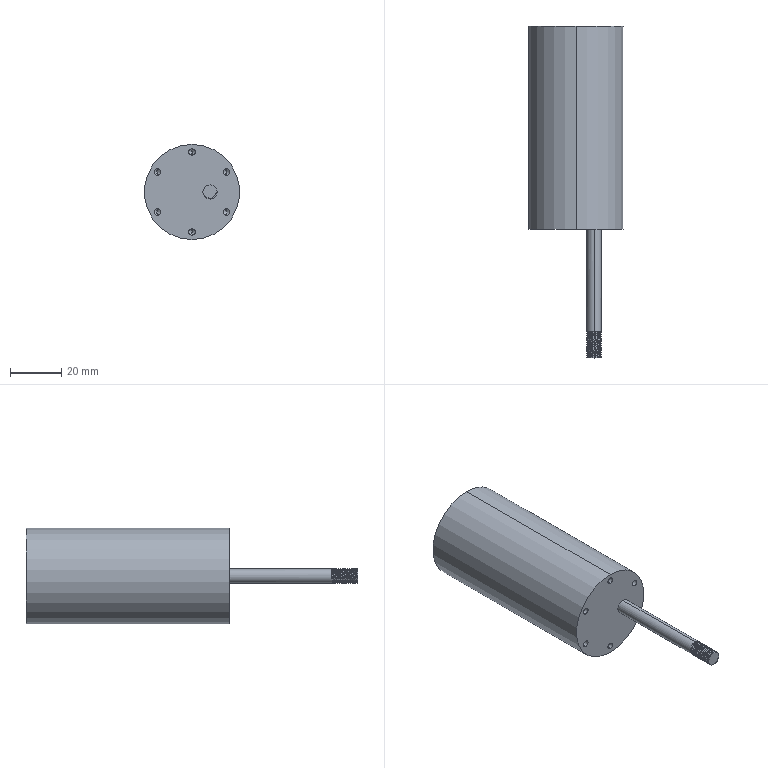Part | SolidWorks | features CirPattern 1, Extrusion 1, HoleWzd 1, ICE 1, SweepThread 1 | 1 solid | 64 faces | box 37 x 129 x 37 mm | volume 85867 mm3 | cylinder 44 | cone 12 | plane 5 | spline 3 | commonest cylinder face diameters 5.5 x30 2.5 x12 37 x2